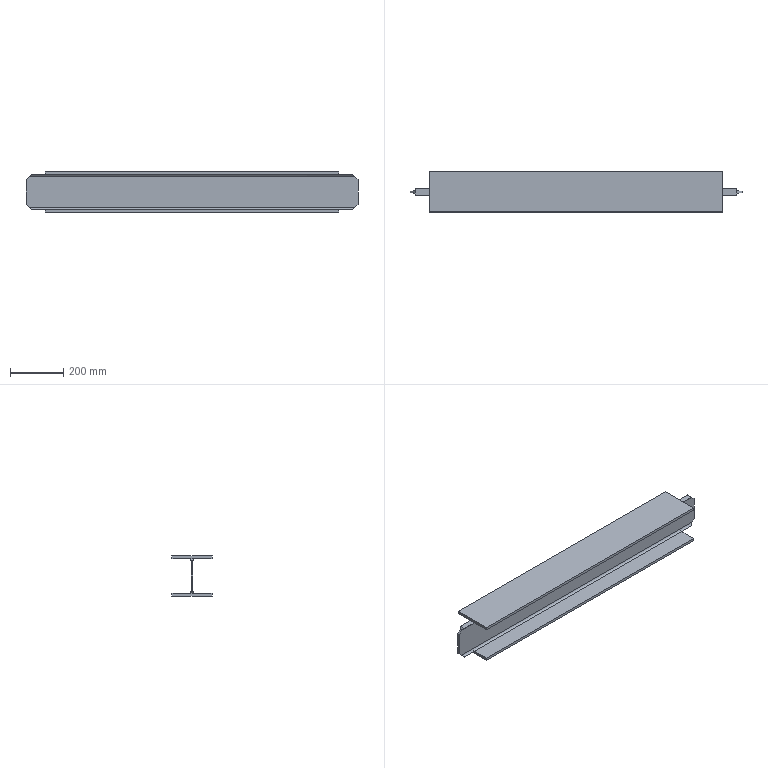Part | STEP file | 02-Longitudinal beam H150X150_default<machining> | 1 solid | 30 faces | box 1243 x 150 x 150 mm | volume 4482817 mm3 | plane 26 | cylinder 4 | commonest cylinder face diameters 16 x4